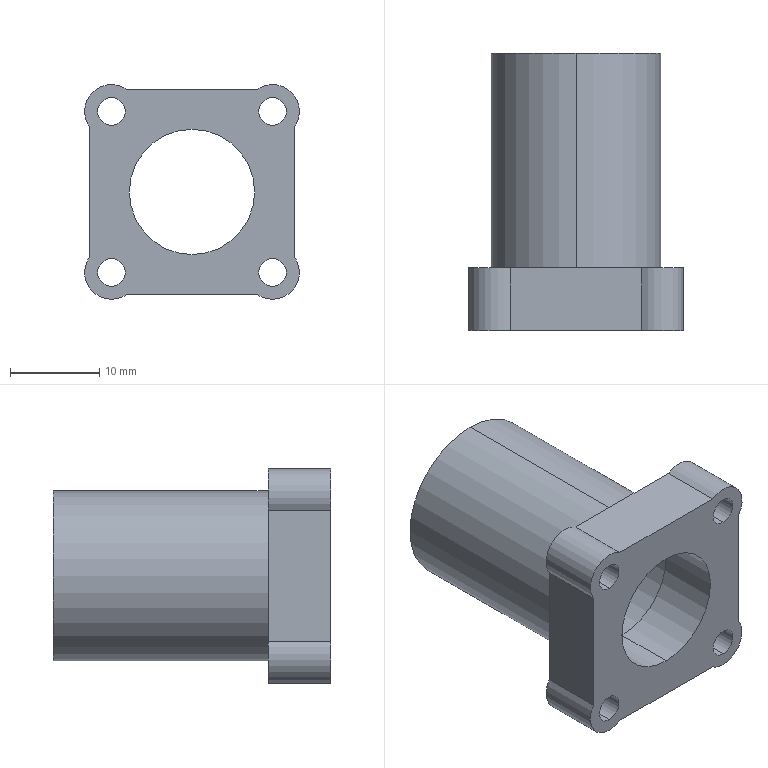Part | SolidWorks | features Extrusion 1, ICE 1 | 1 solid | 28 faces | box 24 x 31 x 24 mm | volume 4448 mm3 | cylinder 20 | plane 8 | commonest cylinder face diameters 3.1 x8 6 x6 14 x2 16 x2 19 x2
STEP:
#1=CARTESIAN_POINT('',(0.,31.,-8.));
#2=VERTEX_POINT('',#1);
#3=CARTESIAN_POINT('',(0.,31.,8.));
#4=VERTEX_POINT('',#3);
#5=CARTESIAN_POINT('',(0.,31.,0.));
#6=DIRECTION('',(0.,1.,0.));
#7=DIRECTION('',(0.,0.,1.));
#8=AXIS2_PLACEMENT_3D('',#5,#6,#7);
#9=CIRCLE('',#8,8.);
#10=EDGE_CURVE('',#2,#4,#9,.T.);
#11=ORIENTED_EDGE('',*,*,#10,.T.);
#12=CARTESIAN_POINT('',(0.,7.,8.));
#13=VERTEX_POINT('',#12);
#14=CARTESIAN_POINT('',(0.,31.,8.));
#15=DIRECTION('',(0.,-1.,0.));
#16=VECTOR('',#15,1000.);
#17=LINE('',#14,#16);
#18=EDGE_CURVE('',#4,#13,#17,.T.);
#19=ORIENTED_EDGE('',*,*,#18,.T.);
#20=CARTESIAN_POINT('',(0.,7.,-8.));
#21=VERTEX_POINT('',#20);
#22=CARTESIAN_POINT('',(0.,7.,0.));
#23=DIRECTION('',(0.,-1.,0.));
#24=DIRECTION('',(0.,0.,1.));
#25=AXIS2_PLACEMENT_3D('',#22,#23,#24);
#26=CIRCLE('',#25,8.);
#27=EDGE_CURVE('',#13,#21,#26,.T.);
#28=ORIENTED_EDGE('',*,*,#27,.T.);
#29=CARTESIAN_POINT('',(0.,31.,-8.));
#30=DIRECTION('',(0.,-1.,0.));
#31=VECTOR('',#30,1000.);
#32=LINE('',#29,#31);
#33=EDGE_CURVE('',#2,#21,#32,.T.);
#34=ORIENTED_EDGE('',*,*,#33,.F.);
#35=EDGE_LOOP('',(#11,#19,#28,#34));
#36=FACE_OUTER_BOUND('',#35,.T.);
#37=CARTESIAN_POINT('',(0.,31.,0.));
#38=DIRECTION('',(0.,-1.,0.));
#39=DIRECTION('',(0.,0.,-1.));
#40=AXIS2_PLACEMENT_3D('',#37,#38,#39);
#41=CYLINDRICAL_SURFACE('',#40,8.);
#42=ADVANCED_FACE('',(#36),#41,.F.);
#43=CARTESIAN_POINT('',(0.,31.,9.5));
#44=VERTEX_POINT('',#43);
#45=CARTESIAN_POINT('',(0.,31.,-9.5));
#46=VERTEX_POINT('',#45);
#47=CARTESIAN_POINT('',(0.,31.,0.));
#48=DIRECTION('',(0.,1.,0.));
#49=DIRECTION('',(0.,0.,1.));
#50=AXIS2_PLACEMENT_3D('',#47,#48,#49);
#51=CIRCLE('',#50,9.5);
#52=EDGE_CURVE('',#44,#46,#51,.T.);
#53=ORIENTED_EDGE('',*,*,#52,.F.);
#54=CARTESIAN_POINT('',(0.,7.,9.5));
#55=VERTEX_POINT('',#54);
#56=CARTESIAN_POINT('',(0.,31.,9.5));
#57=DIRECTION('',(0.,-1.,0.));
#58=VECTOR('',#57,1000.);
#59=LINE('',#56,#58);
#60=EDGE_CURVE('',#44,#55,#59,.T.);
#61=ORIENTED_EDGE('',*,*,#60,.T.);
#62=CARTESIAN_POINT('',(0.,7.,-9.5));
#63=VERTEX_POINT('',#62);
#64=CARTESIAN_POINT('',(0.,7.,0.));
#65=DIRECTION('',(0.,1.,0.));
#66=DIRECTION('',(0.,0.,1.));
#67=AXIS2_PLACEMENT_3D('',#64,#65,#66);
#68=CIRCLE('',#67,9.5);
#69=EDGE_CURVE('',#55,#63,#68,.T.);
#70=ORIENTED_EDGE('',*,*,#69,.T.);
#71=CARTESIAN_POINT('',(0.,31.,-9.5));
#72=DIRECTION('',(0.,-1.,0.));
#73=VECTOR('',#72,1000.);
#74=LINE('',#71,#73);
#75=EDGE_CURVE('',#46,#63,#74,.T.);
#76=ORIENTED_EDGE('',*,*,#75,.F.);
#77=EDGE_LOOP('',(#53,#61,#70,#76));
#78=FACE_OUTER_BOUND('',#77,.T.);
#79=CARTESIAN_POINT('',(0.,31.,0.));
#80=DIRECTION('',(0.,-1.,0.));
#81=DIRECTION('',(0.,0.,-1.));
#82=AXIS2_PLACEMENT_3D('',#79,#80,#81);
#83=CYLINDRICAL_SURFACE('',#82,9.5);
#84=ADVANCED_FACE('',(#78),#83,.T.);
#85=CARTESIAN_POINT('',(9.,7.,7.45));
#86=VERTEX_POINT('',#85);
#87=CARTESIAN_POINT('',(9.,7.,10.55));
#88=VERTEX_POINT('',#87);
#89=CARTESIAN_POINT('',(9.,7.,9.));
#90=DIRECTION('',(0.,1.,0.));
#91=DIRECTION('',(0.,0.,1.));
#92=AXIS2_PLACEMENT_3D('',#89,#90,#91);
#93=CIRCLE('',#92,1.55);
#94=EDGE_CURVE('',#86,#88,#93,.T.);
#95=ORIENTED_EDGE('',*,*,#94,.T.);
#96=CARTESIAN_POINT('',(9.,0.,10.55));
#97=VERTEX_POINT('',#96);
#98=CARTESIAN_POINT('',(9.,7.,10.55));
#99=DIRECTION('',(0.,-1.,0.));
#100=VECTOR('',#99,1000.);
#101=LINE('',#98,#100);
#102=EDGE_CURVE('',#88,#97,#101,.T.);
#103=ORIENTED_EDGE('',*,*,#102,.T.);
#104=CARTESIAN_POINT('',(9.,0.,7.45));
#105=VERTEX_POINT('',#104);
#106=CARTESIAN_POINT('',(9.,0.,9.));
#107=DIRECTION('',(0.,1.,0.));
#108=DIRECTION('',(0.,0.,1.));
#109=AXIS2_PLACEMENT_3D('',#106,#107,#108);
#110=CIRCLE('',#109,1.55);
#111=EDGE_CURVE('',#105,#97,#110,.T.);
#112=ORIENTED_EDGE('',*,*,#111,.F.);
#113=CARTESIAN_POINT('',(9.,7.,7.45));
#114=DIRECTION('',(0.,-1.,0.));
#115=VECTOR('',#114,1000.);
#116=LINE('',#113,#115);
#117=EDGE_CURVE('',#86,#105,#116,.T.);
#118=ORIENTED_EDGE('',*,*,#117,.F.);
#119=EDGE_LOOP('',(#95,#103,#112,#118));
#120=FACE_OUTER_BOUND('',#119,.T.);
#121=CARTESIAN_POINT('',(9.,7.,9.));
#122=DIRECTION('',(0.,-1.,0.));
#123=DIRECTION('',(0.,0.,-1.));
#124=AXIS2_PLACEMENT_3D('',#121,#122,#123);
#125=CYLINDRICAL_SURFACE('',#124,1.55);
#126=ADVANCED_FACE('',(#120),#125,.F.);
#127=CARTESIAN_POINT('',(0.,7.,-7.));
#128=VERTEX_POINT('',#127);
#129=CARTESIAN_POINT('',(0.,7.,7.));
#130=VERTEX_POINT('',#129);
#131=CARTESIAN_POINT('',(0.,7.,0.));
#132=DIRECTION('',(0.,1.,0.));
#133=DIRECTION('',(0.,0.,1.));
#134=AXIS2_PLACEMENT_3D('',#131,#132,#133);
#135=CIRCLE('',#134,7.);
#136=EDGE_CURVE('',#128,#130,#135,.T.);
#137=ORIENTED_EDGE('',*,*,#136,.T.);
#138=CARTESIAN_POINT('',(0.,0.,7.));
#139=VERTEX_POINT('',#138);
#140=CARTESIAN_POINT('',(0.,7.,7.));
#141=DIRECTION('',(0.,-1.,0.));
#142=VECTOR('',#141,1000.);
#143=LINE('',#140,#142);
#144=EDGE_CURVE('',#130,#139,#143,.T.);
#145=ORIENTED_EDGE('',*,*,#144,.T.);
#146=CARTESIAN_POINT('',(0.,0.,-7.));
#147=VERTEX_POINT('',#146);
#148=CARTESIAN_POINT('',(0.,0.,0.));
#149=DIRECTION('',(0.,1.,0.));
#150=DIRECTION('',(0.,0.,1.));
#151=AXIS2_PLACEMENT_3D('',#148,#149,#150);
#152=CIRCLE('',#151,7.);
#153=EDGE_CURVE('',#147,#139,#152,.T.);
#154=ORIENTED_EDGE('',*,*,#153,.F.);
#155=CARTESIAN_POINT('',(0.,7.,-7.));
#156=DIRECTION('',(0.,-1.,0.));
#157=VECTOR('',#156,1000.);
#158=LINE('',#155,#157);
#159=EDGE_CURVE('',#128,#147,#158,.T.);
#160=ORIENTED_EDGE('',*,*,#159,.F.);
#161=EDGE_LOOP('',(#137,#145,#154,#160));
#162=FACE_OUTER_BOUND('',#161,.T.);
#163=CARTESIAN_POINT('',(0.,7.,0.));
#164=DIRECTION('',(0.,-1.,0.));
#165=DIRECTION('',(0.,0.,-1.));
#166=AXIS2_PLACEMENT_3D('',#163,#164,#165);
#167=CYLINDRICAL_SURFACE('',#166,7.);
#168=ADVANCED_FACE('',(#162),#167,.F.);
#169=CARTESIAN_POINT('',(-9.,7.,7.45));
#170=VERTEX_POINT('',#169);
#171=CARTESIAN_POINT('',(-9.,7.,10.55));
#172=VERTEX_POINT('',#171);
#173=CARTESIAN_POINT('',(-9.,7.,9.));
#174=DIRECTION('',(0.,1.,0.));
#175=DIRECTION('',(0.,0.,1.));
#176=AXIS2_PLACEMENT_3D('',#173,#174,#175);
#177=CIRCLE('',#176,1.55);
#178=EDGE_CURVE('',#170,#172,#177,.T.);
#179=ORIENTED_EDGE('',*,*,#178,.T.);
#180=CARTESIAN_POINT('',(-9.,0.,10.55));
#181=VERTEX_POINT('',#180);
#182=CARTESIAN_POINT('',(-9.,7.,10.55));
#183=DIRECTION('',(0.,-1.,0.));
#184=VECTOR('',#183,1000.);
#185=LINE('',#182,#184);
#186=EDGE_CURVE('',#172,#181,#185,.T.);
#187=ORIENTED_EDGE('',*,*,#186,.T.);
#188=CARTESIAN_POINT('',(-9.,0.,7.45));
#189=VERTEX_POINT('',#188);
#190=CARTESIAN_POINT('',(-9.,0.,9.));
#191=DIRECTION('',(0.,1.,0.));
#192=DIRECTION('',(0.,0.,1.));
#193=AXIS2_PLACEMENT_3D('',#190,#191,#192);
#194=CIRCLE('',#193,1.55);
#195=EDGE_CURVE('',#189,#181,#194,.T.);
#196=ORIENTED_EDGE('',*,*,#195,.F.);
#197=CARTESIAN_POINT('',(-9.,7.,7.45));
#198=DIRECTION('',(0.,-1.,0.));
#199=VECTOR('',#198,1000.);
#200=LINE('',#197,#199);
#201=EDGE_CURVE('',#170,#189,#200,.T.);
#202=ORIENTED_EDGE('',*,*,#201,.F.);
#203=EDGE_LOOP('',(#179,#187,#196,#202));
#204=FACE_OUTER_BOUND('',#203,.T.);
#205=CARTESIAN_POINT('',(-9.,7.,9.));
#206=DIRECTION('',(0.,-1.,0.));
#207=DIRECTION('',(0.,0.,-1.));
#208=AXIS2_PLACEMENT_3D('',#205,#206,#207);
#209=CYLINDRICAL_SURFACE('',#208,1.55);
#210=ADVANCED_FACE('',(#204),#209,.F.);
#211=CARTESIAN_POINT('',(-9.,7.,-10.55));
#212=VERTEX_POINT('',#211);
#213=CARTESIAN_POINT('',(-9.,7.,-7.45));
#214=VERTEX_POINT('',#213);
#215=CARTESIAN_POINT('',(-9.,7.,-9.));
#216=DIRECTION('',(0.,1.,0.));
#217=DIRECTION('',(0.,0.,1.));
#218=AXIS2_PLACEMENT_3D('',#215,#216,#217);
#219=CIRCLE('',#218,1.55);
#220=EDGE_CURVE('',#212,#214,#219,.T.);
#221=ORIENTED_EDGE('',*,*,#220,.T.);
#222=CARTESIAN_POINT('',(-9.,0.,-7.45));
#223=VERTEX_POINT('',#222);
#224=CARTESIAN_POINT('',(-9.,7.,-7.45));
#225=DIRECTION('',(0.,-1.,0.));
#226=VECTOR('',#225,1000.);
#227=LINE('',#224,#226);
#228=EDGE_CURVE('',#214,#223,#227,.T.);
#229=ORIENTED_EDGE('',*,*,#228,.T.);
#230=CARTESIAN_POINT('',(-9.,0.,-10.55));
#231=VERTEX_POINT('',#230);
#232=CARTESIAN_POINT('',(-9.,0.,-9.));
#233=DIRECTION('',(0.,1.,0.));
#234=DIRECTION('',(0.,0.,1.));
#235=AXIS2_PLACEMENT_3D('',#232,#233,#234);
#236=CIRCLE('',#235,1.55);
#237=EDGE_CURVE('',#231,#223,#236,.T.);
#238=ORIENTED_EDGE('',*,*,#237,.F.);
#239=CARTESIAN_POINT('',(-9.,7.,-10.55));
#240=DIRECTION('',(0.,-1.,0.));
#241=VECTOR('',#240,1000.);
#242=LINE('',#239,#241);
#243=EDGE_CURVE('',#212,#231,#242,.T.);
#244=ORIENTED_EDGE('',*,*,#243,.F.);
#245=EDGE_LOOP('',(#221,#229,#238,#244));
#246=FACE_OUTER_BOUND('',#245,.T.);
#247=CARTESIAN_POINT('',(-9.,7.,-9.));
#248=DIRECTION('',(0.,-1.,0.));
#249=DIRECTION('',(0.,0.,-1.));
#250=AXIS2_PLACEMENT_3D('',#247,#248,#249);
#251=CYLINDRICAL_SURFACE('',#250,1.55);
#252=ADVANCED_FACE('',(#246),#251,.F.);
#253=CARTESIAN_POINT('',(9.,7.,-10.55));
#254=VERTEX_POINT('',#253);
#255=CARTESIAN_POINT('',(9.,7.,-7.45));
#256=VERTEX_POINT('',#255);
#257=CARTESIAN_POINT('',(9.,7.,-9.));
#258=DIRECTION('',(0.,1.,0.));
#259=DIRECTION('',(0.,0.,1.));
#260=AXIS2_PLACEMENT_3D('',#257,#258,#259);
#261=CIRCLE('',#260,1.55);
#262=EDGE_CURVE('',#254,#256,#261,.T.);
#263=ORIENTED_EDGE('',*,*,#262,.T.);
#264=CARTESIAN_POINT('',(9.,0.,-7.45));
#265=VERTEX_POINT('',#264);
#266=CARTESIAN_POINT('',(9.,7.,-7.45));
#267=DIRECTION('',(0.,-1.,0.));
#268=VECTOR('',#267,1000.);
#269=LINE('',#266,#268);
#270=EDGE_CURVE('',#256,#265,#269,.T.);
#271=ORIENTED_EDGE('',*,*,#270,.T.);
#272=CARTESIAN_POINT('',(9.,0.,-10.55));
#273=VERTEX_POINT('',#272);
#274=CARTESIAN_POINT('',(9.,0.,-9.));
#275=DIRECTION('',(0.,1.,0.));
#276=DIRECTION('',(0.,0.,1.));
#277=AXIS2_PLACEMENT_3D('',#274,#275,#276);
#278=CIRCLE('',#277,1.55);
#279=EDGE_CURVE('',#273,#265,#278,.T.);
#280=ORIENTED_EDGE('',*,*,#279,.F.);
#281=CARTESIAN_POINT('',(9.,7.,-10.55));
#282=DIRECTION('',(0.,-1.,0.));
#283=VECTOR('',#282,1000.);
#284=LINE('',#281,#283);
#285=EDGE_CURVE('',#254,#273,#284,.T.);
#286=ORIENTED_EDGE('',*,*,#285,.F.);
#287=EDGE_LOOP('',(#263,#271,#280,#286));
#288=FACE_OUTER_BOUND('',#287,.T.);
#289=CARTESIAN_POINT('',(9.,7.,-9.));
#290=DIRECTION('',(0.,-1.,0.));
#291=DIRECTION('',(0.,0.,-1.));
#292=AXIS2_PLACEMENT_3D('',#289,#290,#291);
#293=CYLINDRICAL_SURFACE('',#292,1.55);
#294=ADVANCED_FACE('',(#288),#293,.F.);
#295=CARTESIAN_POINT('',(-9.,7.,-12.));
#296=VERTEX_POINT('',#295);
#297=CARTESIAN_POINT('',(-11.5,7.,-7.342));
#298=VERTEX_POINT('',#297);
#299=CARTESIAN_POINT('',(-9.,7.,-9.));
#300=DIRECTION('',(0.,1.,0.));
#301=DIRECTION('',(0.,0.,1.));
#302=AXIS2_PLACEMENT_3D('',#299,#300,#301);
#303=CIRCLE('',#302,3.);
#304=EDGE_CURVE('',#296,#298,#303,.T.);
#305=ORIENTED_EDGE('',*,*,#304,.F.);
#306=CARTESIAN_POINT('',(-9.,0.,-12.));
#307=VERTEX_POINT('',#306);
#308=CARTESIAN_POINT('',(-9.,7.,-12.));
#309=DIRECTION('',(0.,-1.,0.));
#310=VECTOR('',#309,1000.);
#311=LINE('',#308,#310);
#312=EDGE_CURVE('',#296,#307,#311,.T.);
#313=ORIENTED_EDGE('',*,*,#312,.T.);
#314=CARTESIAN_POINT('',(-11.5,0.,-7.342));
#315=VERTEX_POINT('',#314);
#316=CARTESIAN_POINT('',(-9.,0.,-9.));
#317=DIRECTION('',(0.,1.,0.));
#318=DIRECTION('',(0.,0.,1.));
#319=AXIS2_PLACEMENT_3D('',#316,#317,#318);
#320=CIRCLE('',#319,3.);
#321=EDGE_CURVE('',#307,#315,#320,.T.);
#322=ORIENTED_EDGE('',*,*,#321,.T.);
#323=CARTESIAN_POINT('',(-11.5,7.,-7.342));
#324=DIRECTION('',(0.,-1.,0.));
#325=VECTOR('',#324,1000.);
#326=LINE('',#323,#325);
#327=EDGE_CURVE('',#298,#315,#326,.T.);
#328=ORIENTED_EDGE('',*,*,#327,.F.);
#329=EDGE_LOOP('',(#305,#313,#322,#328));
#330=FACE_OUTER_BOUND('',#329,.T.);
#331=CARTESIAN_POINT('',(-9.,7.,-9.));
#332=DIRECTION('',(0.,-1.,0.));
#333=DIRECTION('',(0.,0.,-1.));
#334=AXIS2_PLACEMENT_3D('',#331,#332,#333);
#335=CYLINDRICAL_SURFACE('',#334,3.);
#336=ADVANCED_FACE('',(#330),#335,.T.);
#337=CARTESIAN_POINT('',(9.,7.,-12.));
#338=VERTEX_POINT('',#337);
#339=CARTESIAN_POINT('',(7.342,7.,-11.5));
#340=VERTEX_POINT('',#339);
#341=CARTESIAN_POINT('',(9.,7.,-9.));
#342=DIRECTION('',(0.,1.,0.));
#343=DIRECTION('',(0.,0.,1.));
#344=AXIS2_PLACEMENT_3D('',#341,#342,#343);
#345=CIRCLE('',#344,3.);
#346=EDGE_CURVE('',#338,#340,#345,.T.);
#347=ORIENTED_EDGE('',*,*,#346,.F.);
#348=CARTESIAN_POINT('',(9.,0.,-12.));
#349=VERTEX_POINT('',#348);
#350=CARTESIAN_POINT('',(9.,7.,-12.));
#351=DIRECTION('',(0.,-1.,0.));
#352=VECTOR('',#351,1000.);
#353=LINE('',#350,#352);
#354=EDGE_CURVE('',#338,#349,#353,.T.);
#355=ORIENTED_EDGE('',*,*,#354,.T.);
#356=CARTESIAN_POINT('',(7.342,0.,-11.5));
#357=VERTEX_POINT('',#356);
#358=CARTESIAN_POINT('',(9.,0.,-9.));
#359=DIRECTION('',(0.,1.,0.));
#360=DIRECTION('',(0.,0.,1.));
#361=AXIS2_PLACEMENT_3D('',#358,#359,#360);
#362=CIRCLE('',#361,3.);
#363=EDGE_CURVE('',#349,#357,#362,.T.);
#364=ORIENTED_EDGE('',*,*,#363,.T.);
#365=CARTESIAN_POINT('',(7.342,7.,-11.5));
#366=DIRECTION('',(0.,-1.,0.));
#367=VECTOR('',#366,1000.);
#368=LINE('',#365,#367);
#369=EDGE_CURVE('',#340,#357,#368,.T.);
#370=ORIENTED_EDGE('',*,*,#369,.F.);
#371=EDGE_LOOP('',(#347,#355,#364,#370));
#372=FACE_OUTER_BOUND('',#371,.T.);
#373=CARTESIAN_POINT('',(9.,7.,-9.));
#374=DIRECTION('',(0.,-1.,0.));
#375=DIRECTION('',(0.,0.,-1.));
#376=AXIS2_PLACEMENT_3D('',#373,#374,#375);
#377=CYLINDRICAL_SURFACE('',#376,3.);
#378=ADVANCED_FACE('',(#372),#377,.T.);
#379=ORIENTED_EDGE('',*,*,#136,.F.);
#380=CARTESIAN_POINT('',(0.,7.,0.));
#381=DIRECTION('',(0.,1.,0.));
#382=DIRECTION('',(0.,0.,1.));
#383=AXIS2_PLACEMENT_3D('',#380,#381,#382);
#384=CIRCLE('',#383,7.);
#385=EDGE_CURVE('',#130,#128,#384,.T.);
#386=ORIENTED_EDGE('',*,*,#385,.F.);
#387=EDGE_LOOP('',(#379,#386));
#388=FACE_BOUND('',#387,.T.);
#389=CARTESIAN_POINT('',(0.,7.,0.));
#390=DIRECTION('',(0.,-1.,0.));
#391=DIRECTION('',(0.,0.,1.));
#392=AXIS2_PLACEMENT_3D('',#389,#390,#391);
#393=CIRCLE('',#392,8.);
#394=EDGE_CURVE('',#21,#13,#393,.T.);
#395=ORIENTED_EDGE('',*,*,#394,.F.);
#396=ORIENTED_EDGE('',*,*,#27,.F.);
#397=EDGE_LOOP('',(#395,#396));
#398=FACE_OUTER_BOUND('',#397,.T.);
#399=CARTESIAN_POINT('',(0.,7.,0.));
#400=DIRECTION('',(0.,1.,0.));
#401=DIRECTION('',(0.,0.,1.));
#402=AXIS2_PLACEMENT_3D('',#399,#400,#401);
#403=PLANE('',#402);
#404=ADVANCED_FACE('',(#388,#398),#403,.T.);
#405=CARTESIAN_POINT('',(7.342,0.,11.5));
#406=VERTEX_POINT('',#405);
#407=CARTESIAN_POINT('',(-7.342,0.,11.5));
#408=VERTEX_POINT('',#407);
#409=CARTESIAN_POINT('',(0.,0.,11.5));
#410=DIRECTION('',(-1.,0.,0.));
#411=VECTOR('',#410,1000.);
#412=LINE('',#409,#411);
#413=EDGE_CURVE('',#406,#408,#412,.T.);
#414=ORIENTED_EDGE('',*,*,#413,.F.);
#415=CARTESIAN_POINT('',(7.342,7.,11.5));
#416=VERTEX_POINT('',#415);
#417=CARTESIAN_POINT('',(7.342,7.,11.5));
#418=DIRECTION('',(0.,-1.,0.));
#419=VECTOR('',#418,1000.);
#420=LINE('',#417,#419);
#421=EDGE_CURVE('',#416,#406,#420,.T.);
#422=ORIENTED_EDGE('',*,*,#421,.F.);
#423=CARTESIAN_POINT('',(-7.342,7.,11.5));
#424=VERTEX_POINT('',#423);
#425=CARTESIAN_POINT('',(0.,7.,11.5));
#426=DIRECTION('',(-1.,0.,0.));
#427=VECTOR('',#426,1000.);
#428=LINE('',#425,#427);
#429=EDGE_CURVE('',#416,#424,#428,.T.);
#430=ORIENTED_EDGE('',*,*,#429,.T.);
#431=CARTESIAN_POINT('',(-7.342,7.,11.5));
#432=DIRECTION('',(0.,-1.,0.));
#433=VECTOR('',#432,1000.);
#434=LINE('',#431,#433);
#435=EDGE_CURVE('',#424,#408,#434,.T.);
#436=ORIENTED_EDGE('',*,*,#435,.T.);
#437=EDGE_LOOP('',(#414,#422,#430,#436));
#438=FACE_OUTER_BOUND('',#437,.T.);
#439=CARTESIAN_POINT('',(0.,7.,11.5));
#440=DIRECTION('',(0.,0.,1.));
#441=DIRECTION('',(1.,0.,0.));
#442=AXIS2_PLACEMENT_3D('',#439,#440,#441);
#443=PLANE('',#442);
#444=ADVANCED_FACE('',(#438),#443,.T.);
#445=CARTESIAN_POINT('',(11.5,0.,7.342));
#446=VERTEX_POINT('',#445);
#447=CARTESIAN_POINT('',(9.,0.,9.));
#448=DIRECTION('',(0.,1.,0.));
#449=DIRECTION('',(0.,0.,1.));
#450=AXIS2_PLACEMENT_3D('',#447,#448,#449);
#451=CIRCLE('',#450,3.);
#452=EDGE_CURVE('',#406,#446,#451,.T.);
#453=ORIENTED_EDGE('',*,*,#452,.T.);
#454=CARTESIAN_POINT('',(11.5,7.,7.342));
#455=VERTEX_POINT('',#454);
#456=CARTESIAN_POINT('',(11.5,7.,7.342));
#457=DIRECTION('',(0.,-1.,0.));
#458=VECTOR('',#457,1000.);
#459=LINE('',#456,#458);
#460=EDGE_CURVE('',#455,#446,#459,.T.);
#461=ORIENTED_EDGE('',*,*,#460,.F.);
#462=CARTESIAN_POINT('',(9.,7.,9.));
#463=DIRECTION('',(0.,1.,0.));
#464=DIRECTION('',(0.,0.,1.));
#465=AXIS2_PLACEMENT_3D('',#462,#463,#464);
#466=CIRCLE('',#465,3.);
#467=EDGE_CURVE('',#416,#455,#466,.T.);
#468=ORIENTED_EDGE('',*,*,#467,.F.);
#469=ORIENTED_EDGE('',*,*,#421,.T.);
#470=EDGE_LOOP('',(#453,#461,#468,#469));
#471=FACE_OUTER_BOUND('',#470,.T.);
#472=CARTESIAN_POINT('',(9.,7.,9.));
#473=DIRECTION('',(0.,-1.,0.));
#474=DIRECTION('',(0.,0.,-1.));
#475=AXIS2_PLACEMENT_3D('',#472,#473,#474);
#476=CYLINDRICAL_SURFACE('',#475,3.);
#477=ADVANCED_FACE('',(#471),#476,.T.);
#478=CARTESIAN_POINT('',(11.5,0.,-7.342));
#479=VERTEX_POINT('',#478);
#480=CARTESIAN_POINT('',(11.5,0.,0.));
#481=DIRECTION('',(0.,0.,-1.));
#482=VECTOR('',#481,1000.);
#483=LINE('',#480,#482);
#484=EDGE_CURVE('',#446,#479,#483,.T.);
#485=ORIENTED_EDGE('',*,*,#484,.T.);
#486=CARTESIAN_POINT('',(11.5,7.,-7.342));
#487=VERTEX_POINT('',#486);
#488=CARTESIAN_POINT('',(11.5,7.,-7.342));
#489=DIRECTION('',(0.,-1.,0.));
#490=VECTOR('',#489,1000.);
#491=LINE('',#488,#490);
#492=EDGE_CURVE('',#487,#479,#491,.T.);
#493=ORIENTED_EDGE('',*,*,#492,.F.);
#494=CARTESIAN_POINT('',(11.5,7.,0.));
#495=DIRECTION('',(0.,0.,-1.));
#496=VECTOR('',#495,1000.);
#497=LINE('',#494,#496);
#498=EDGE_CURVE('',#455,#487,#497,.T.);
#499=ORIENTED_EDGE('',*,*,#498,.F.);
#500=ORIENTED_EDGE('',*,*,#460,.T.);
#501=EDGE_LOOP('',(#485,#493,#499,#500));
#502=FACE_OUTER_BOUND('',#501,.T.);
#503=CARTESIAN_POINT('',(11.5,7.,0.));
#504=DIRECTION('',(-1.,0.,0.));
#505=DIRECTION('',(0.,0.,1.));
#506=AXIS2_PLACEMENT_3D('',#503,#504,#505);
#507=PLANE('',#506);
#508=ADVANCED_FACE('',(#502),#507,.F.);
#509=ORIENTED_EDGE('',*,*,#354,.F.);
#510=CARTESIAN_POINT('',(9.,7.,-9.));
#511=DIRECTION('',(0.,1.,0.));
#512=DIRECTION('',(0.,0.,1.));
#513=AXIS2_PLACEMENT_3D('',#510,#511,#512);
#514=CIRCLE('',#513,3.);
#515=EDGE_CURVE('',#487,#338,#514,.T.);
#516=ORIENTED_EDGE('',*,*,#515,.F.);
#517=ORIENTED_EDGE('',*,*,#492,.T.);
#518=CARTESIAN_POINT('',(9.,0.,-9.));
#519=DIRECTION('',(0.,1.,0.));
#520=DIRECTION('',(0.,0.,1.));
#521=AXIS2_PLACEMENT_3D('',#518,#519,#520);
#522=CIRCLE('',#521,3.);
#523=EDGE_CURVE('',#479,#349,#522,.T.);
#524=ORIENTED_EDGE('',*,*,#523,.T.);
#525=EDGE_LOOP('',(#509,#516,#517,#524));
#526=FACE_OUTER_BOUND('',#525,.T.);
#527=CARTESIAN_POINT('',(9.,7.,-9.));
#528=DIRECTION('',(0.,-1.,0.));
#529=DIRECTION('',(0.,0.,-1.));
#530=AXIS2_PLACEMENT_3D('',#527,#528,#529);
#531=CYLINDRICAL_SURFACE('',#530,3.);
#532=ADVANCED_FACE('',(#526),#531,.T.);
#533=CARTESIAN_POINT('',(-7.342,0.,-11.5));
#534=VERTEX_POINT('',#533);
#535=CARTESIAN_POINT('',(0.,0.,-11.5));
#536=DIRECTION('',(1.,0.,0.));
#537=VECTOR('',#536,1000.);
#538=LINE('',#535,#537);
#539=EDGE_CURVE('',#534,#357,#538,.T.);
#540=ORIENTED_EDGE('',*,*,#539,.F.);
#541=CARTESIAN_POINT('',(-7.342,7.,-11.5));
#542=VERTEX_POINT('',#541);
#543=CARTESIAN_POINT('',(-7.342,7.,-11.5));
#544=DIRECTION('',(0.,-1.,0.));
#545=VECTOR('',#544,1000.);
#546=LINE('',#543,#545);
#547=EDGE_CURVE('',#542,#534,#546,.T.);
#548=ORIENTED_EDGE('',*,*,#547,.F.);
#549=CARTESIAN_POINT('',(0.,7.,-11.5));
#550=DIRECTION('',(1.,0.,0.));
#551=VECTOR('',#550,1000.);
#552=LINE('',#549,#551);
#553=EDGE_CURVE('',#542,#340,#552,.T.);
#554=ORIENTED_EDGE('',*,*,#553,.T.);
#555=ORIENTED_EDGE('',*,*,#369,.T.);
#556=EDGE_LOOP('',(#540,#548,#554,#555));
#557=FACE_OUTER_BOUND('',#556,.T.);
#558=CARTESIAN_POINT('',(0.,7.,-11.5));
#559=DIRECTION('',(0.,0.,-1.));
#560=DIRECTION('',(-1.,0.,0.));
#561=AXIS2_PLACEMENT_3D('',#558,#559,#560);
#562=PLANE('',#561);
#563=ADVANCED_FACE('',(#557),#562,.T.);
#564=ORIENTED_EDGE('',*,*,#312,.F.);
#565=CARTESIAN_POINT('',(-9.,7.,-9.));
#566=DIRECTION('',(0.,1.,0.));
#567=DIRECTION('',(0.,0.,1.));
#568=AXIS2_PLACEMENT_3D('',#565,#566,#567);
#569=CIRCLE('',#568,3.);
#570=EDGE_CURVE('',#542,#296,#569,.T.);
#571=ORIENTED_EDGE('',*,*,#570,.F.);
#572=ORIENTED_EDGE('',*,*,#547,.T.);
#573=CARTESIAN_POINT('',(-9.,0.,-9.));
#574=DIRECTION('',(0.,1.,0.));
#575=DIRECTION('',(0.,0.,1.));
#576=AXIS2_PLACEMENT_3D('',#573,#574,#575);
#577=CIRCLE('',#576,3.);
#578=EDGE_CURVE('',#534,#307,#577,.T.);
#579=ORIENTED_EDGE('',*,*,#578,.T.);
#580=EDGE_LOOP('',(#564,#571,#572,#579));
#581=FACE_OUTER_BOUND('',#580,.T.);
#582=CARTESIAN_POINT('',(-9.,7.,-9.));
#583=DIRECTION('',(0.,-1.,0.));
#584=DIRECTION('',(0.,0.,-1.));
#585=AXIS2_PLACEMENT_3D('',#582,#583,#584);
#586=CYLINDRICAL_SURFACE('',#585,3.);
#587=ADVANCED_FACE('',(#581),#586,.T.);
#588=CARTESIAN_POINT('',(-11.5,0.,7.342));
#589=VERTEX_POINT('',#588);
#590=CARTESIAN_POINT('',(-11.5,0.,0.));
#591=DIRECTION('',(0.,0.,1.));
#592=VECTOR('',#591,1000.);
#593=LINE('',#590,#592);
#594=EDGE_CURVE('',#315,#589,#593,.T.);
#595=ORIENTED_EDGE('',*,*,#594,.T.);
#596=CARTESIAN_POINT('',(-11.5,7.,7.342));
#597=VERTEX_POINT('',#596);
#598=CARTESIAN_POINT('',(-11.5,7.,7.342));
#599=DIRECTION('',(0.,-1.,0.));
#600=VECTOR('',#599,1000.);
#601=LINE('',#598,#600);
#602=EDGE_CURVE('',#597,#589,#601,.T.);
#603=ORIENTED_EDGE('',*,*,#602,.F.);
#604=CARTESIAN_POINT('',(-11.5,7.,0.));
#605=DIRECTION('',(0.,0.,1.));
#606=VECTOR('',#605,1000.);
#607=LINE('',#604,#606);
#608=EDGE_CURVE('',#298,#597,#607,.T.);
#609=ORIENTED_EDGE('',*,*,#608,.F.);
#610=ORIENTED_EDGE('',*,*,#327,.T.);
#611=EDGE_LOOP('',(#595,#603,#609,#610));
#612=FACE_OUTER_BOUND('',#611,.T.);
#613=CARTESIAN_POINT('',(-11.5,7.,0.));
#614=DIRECTION('',(1.,0.,0.));
#615=DIRECTION('',(0.,0.,-1.));
#616=AXIS2_PLACEMENT_3D('',#613,#614,#615);
#617=PLANE('',#616);
#618=ADVANCED_FACE('',(#612),#617,.F.);
#619=ORIENTED_EDGE('',*,*,#270,.F.);
#620=CARTESIAN_POINT('',(9.,7.,-9.));
#621=DIRECTION('',(0.,1.,0.));
#622=DIRECTION('',(0.,0.,1.));
#623=AXIS2_PLACEMENT_3D('',#620,#621,#622);
#624=CIRCLE('',#623,1.55);
#625=EDGE_CURVE('',#256,#254,#624,.T.);
#626=ORIENTED_EDGE('',*,*,#625,.T.);
#627=ORIENTED_EDGE('',*,*,#285,.T.);
#628=CARTESIAN_POINT('',(9.,0.,-9.));
#629=DIRECTION('',(0.,1.,0.));
#630=DIRECTION('',(0.,0.,1.));
#631=AXIS2_PLACEMENT_3D('',#628,#629,#630);
#632=CIRCLE('',#631,1.55);
#633=EDGE_CURVE('',#265,#273,#632,.T.);
#634=ORIENTED_EDGE('',*,*,#633,.F.);
#635=EDGE_LOOP('',(#619,#626,#627,#634));
#636=FACE_OUTER_BOUND('',#635,.T.);
#637=CARTESIAN_POINT('',(9.,7.,-9.));
#638=DIRECTION('',(0.,-1.,0.));
#639=DIRECTION('',(0.,0.,-1.));
#640=AXIS2_PLACEMENT_3D('',#637,#638,#639);
#641=CYLINDRICAL_SURFACE('',#640,1.55);
#642=ADVANCED_FACE('',(#636),#641,.F.);
#643=ORIENTED_EDGE('',*,*,#228,.F.);
#644=CARTESIAN_POINT('',(-9.,7.,-9.));
#645=DIRECTION('',(0.,1.,0.));
#646=DIRECTION('',(0.,0.,1.));
#647=AXIS2_PLACEMENT_3D('',#644,#645,#646);
#648=CIRCLE('',#647,1.55);
#649=EDGE_CURVE('',#214,#212,#648,.T.);
#650=ORIENTED_EDGE('',*,*,#649,.T.);
#651=ORIENTED_EDGE('',*,*,#243,.T.);
#652=CARTESIAN_POINT('',(-9.,0.,-9.));
#653=DIRECTION('',(0.,1.,0.));
#654=DIRECTION('',(0.,0.,1.));
#655=AXIS2_PLACEMENT_3D('',#652,#653,#654);
#656=CIRCLE('',#655,1.55);
#657=EDGE_CURVE('',#223,#231,#656,.T.);
#658=ORIENTED_EDGE('',*,*,#657,.F.);
#659=EDGE_LOOP('',(#643,#650,#651,#658));
#660=FACE_OUTER_BOUND('',#659,.T.);
#661=CARTESIAN_POINT('',(-9.,7.,-9.));
#662=DIRECTION('',(0.,-1.,0.));
#663=DIRECTION('',(0.,0.,-1.));
#664=AXIS2_PLACEMENT_3D('',#661,#662,#663);
#665=CYLINDRICAL_SURFACE('',#664,1.55);
#666=ADVANCED_FACE('',(#660),#665,.F.);
#667=ORIENTED_EDGE('',*,*,#186,.F.);
#668=CARTESIAN_POINT('',(-9.,7.,9.));
#669=DIRECTION('',(0.,1.,0.));
#670=DIRECTION('',(0.,0.,1.));
#671=AXIS2_PLACEMENT_3D('',#668,#669,#670);
#672=CIRCLE('',#671,1.55);
#673=EDGE_CURVE('',#172,#170,#672,.T.);
#674=ORIENTED_EDGE('',*,*,#673,.T.);
#675=ORIENTED_EDGE('',*,*,#201,.T.);
#676=CARTESIAN_POINT('',(-9.,0.,9.));
#677=DIRECTION('',(0.,1.,0.));
#678=DIRECTION('',(0.,0.,1.));
#679=AXIS2_PLACEMENT_3D('',#676,#677,#678);
#680=CIRCLE('',#679,1.55);
#681=EDGE_CURVE('',#181,#189,#680,.T.);
#682=ORIENTED_EDGE('',*,*,#681,.F.);
#683=EDGE_LOOP('',(#667,#674,#675,#682));
#684=FACE_OUTER_BOUND('',#683,.T.);
#685=CARTESIAN_POINT('',(-9.,7.,9.));
#686=DIRECTION('',(0.,-1.,0.));
#687=DIRECTION('',(0.,0.,-1.));
#688=AXIS2_PLACEMENT_3D('',#685,#686,#687);
#689=CYLINDRICAL_SURFACE('',#688,1.55);
#690=ADVANCED_FACE('',(#684),#689,.F.);
#691=CARTESIAN_POINT('',(-9.,0.,9.));
#692=DIRECTION('',(0.,1.,0.));
#693=DIRECTION('',(0.,0.,1.));
#694=AXIS2_PLACEMENT_3D('',#691,#692,#693);
#695=CIRCLE('',#694,3.);
#696=EDGE_CURVE('',#589,#408,#695,.T.);
#697=ORIENTED_EDGE('',*,*,#696,.T.);
#698=ORIENTED_EDGE('',*,*,#435,.F.);
#699=CARTESIAN_POINT('',(-9.,7.,9.));
#700=DIRECTION('',(0.,1.,0.));
#701=DIRECTION('',(0.,0.,1.));
#702=AXIS2_PLACEMENT_3D('',#699,#700,#701);
#703=CIRCLE('',#702,3.);
#704=EDGE_CURVE('',#597,#424,#703,.T.);
#705=ORIENTED_EDGE('',*,*,#704,.F.);
#706=ORIENTED_EDGE('',*,*,#602,.T.);
#707=EDGE_LOOP('',(#697,#698,#705,#706));
#708=FACE_OUTER_BOUND('',#707,.T.);
#709=CARTESIAN_POINT('',(-9.,7.,9.));
#710=DIRECTION('',(0.,-1.,0.));
#711=DIRECTION('',(0.,0.,-1.));
#712=AXIS2_PLACEMENT_3D('',#709,#710,#711);
#713=CYLINDRICAL_SURFACE('',#712,3.);
#714=ADVANCED_FACE('',(#708),#713,.T.);
#715=ORIENTED_EDGE('',*,*,#144,.F.);
#716=ORIENTED_EDGE('',*,*,#385,.T.);
#717=ORIENTED_EDGE('',*,*,#159,.T.);
#718=CARTESIAN_POINT('',(0.,0.,0.));
#719=DIRECTION('',(0.,1.,0.));
#720=DIRECTION('',(0.,0.,1.));
#721=AXIS2_PLACEMENT_3D('',#718,#719,#720);
#722=CIRCLE('',#721,7.);
#723=EDGE_CURVE('',#139,#147,#722,.T.);
#724=ORIENTED_EDGE('',*,*,#723,.F.);
#725=EDGE_LOOP('',(#715,#716,#717,#724));
#726=FACE_OUTER_BOUND('',#725,.T.);
#727=CARTESIAN_POINT('',(0.,7.,0.));
#728=DIRECTION('',(0.,-1.,0.));
#729=DIRECTION('',(0.,0.,-1.));
#730=AXIS2_PLACEMENT_3D('',#727,#728,#729);
#731=CYLINDRICAL_SURFACE('',#730,7.);
#732=ADVANCED_FACE('',(#726),#731,.F.);
#733=ORIENTED_EDGE('',*,*,#102,.F.);
#734=CARTESIAN_POINT('',(9.,7.,9.));
#735=DIRECTION('',(0.,1.,0.));
#736=DIRECTION('',(0.,0.,1.));
#737=AXIS2_PLACEMENT_3D('',#734,#735,#736);
#738=CIRCLE('',#737,1.55);
#739=EDGE_CURVE('',#88,#86,#738,.T.);
#740=ORIENTED_EDGE('',*,*,#739,.T.);
#741=ORIENTED_EDGE('',*,*,#117,.T.);
#742=CARTESIAN_POINT('',(9.,0.,9.));
#743=DIRECTION('',(0.,1.,0.));
#744=DIRECTION('',(0.,0.,1.));
#745=AXIS2_PLACEMENT_3D('',#742,#743,#744);
#746=CIRCLE('',#745,1.55);
#747=EDGE_CURVE('',#97,#105,#746,.T.);
#748=ORIENTED_EDGE('',*,*,#747,.F.);
#749=EDGE_LOOP('',(#733,#740,#741,#748));
#750=FACE_OUTER_BOUND('',#749,.T.);
#751=CARTESIAN_POINT('',(9.,7.,9.));
#752=DIRECTION('',(0.,-1.,0.));
#753=DIRECTION('',(0.,0.,-1.));
#754=AXIS2_PLACEMENT_3D('',#751,#752,#753);
#755=CYLINDRICAL_SURFACE('',#754,1.55);
#756=ADVANCED_FACE('',(#750),#755,.F.);
#757=CARTESIAN_POINT('',(0.,7.,0.));
#758=DIRECTION('',(0.,1.,0.));
#759=DIRECTION('',(0.,0.,1.));
#760=AXIS2_PLACEMENT_3D('',#757,#758,#759);
#761=CIRCLE('',#760,9.5);
#762=EDGE_CURVE('',#63,#55,#761,.T.);
#763=ORIENTED_EDGE('',*,*,#762,.F.);
#764=ORIENTED_EDGE('',*,*,#69,.F.);
#765=EDGE_LOOP('',(#763,#764));
#766=FACE_BOUND('',#765,.T.);
#767=ORIENTED_EDGE('',*,*,#429,.F.);
#768=ORIENTED_EDGE('',*,*,#467,.T.);
#769=ORIENTED_EDGE('',*,*,#498,.T.);
#770=ORIENTED_EDGE('',*,*,#515,.T.);
#771=ORIENTED_EDGE('',*,*,#346,.T.);
#772=ORIENTED_EDGE('',*,*,#553,.F.);
#773=ORIENTED_EDGE('',*,*,#570,.T.);
#774=ORIENTED_EDGE('',*,*,#304,.T.);
#775=ORIENTED_EDGE('',*,*,#608,.T.);
#776=ORIENTED_EDGE('',*,*,#704,.T.);
#777=EDGE_LOOP('',(#767,#768,#769,#770,#771,#772,#773,#774,#775,#776));
#778=FACE_OUTER_BOUND('',#777,.T.);
#779=ORIENTED_EDGE('',*,*,#178,.F.);
#780=ORIENTED_EDGE('',*,*,#673,.F.);
#781=EDGE_LOOP('',(#779,#780));
#782=FACE_BOUND('',#781,.T.);
#783=ORIENTED_EDGE('',*,*,#220,.F.);
#784=ORIENTED_EDGE('',*,*,#649,.F.);
#785=EDGE_LOOP('',(#783,#784));
#786=FACE_BOUND('',#785,.T.);
#787=ORIENTED_EDGE('',*,*,#262,.F.);
#788=ORIENTED_EDGE('',*,*,#625,.F.);
#789=EDGE_LOOP('',(#787,#788));
#790=FACE_BOUND('',#789,.T.);
#791=ORIENTED_EDGE('',*,*,#94,.F.);
#792=ORIENTED_EDGE('',*,*,#739,.F.);
#793=EDGE_LOOP('',(#791,#792));
#794=FACE_BOUND('',#793,.T.);
#795=CARTESIAN_POINT('',(0.,7.,0.));
#796=DIRECTION('',(0.,1.,0.));
#797=DIRECTION('',(0.,0.,1.));
#798=AXIS2_PLACEMENT_3D('',#795,#796,#797);
#799=PLANE('',#798);
#800=ADVANCED_FACE('',(#766,#778,#782,#786,#790,#794),#799,.T.);
#801=ORIENTED_EDGE('',*,*,#153,.T.);
#802=ORIENTED_EDGE('',*,*,#723,.T.);
#803=EDGE_LOOP('',(#801,#802));
#804=FACE_BOUND('',#803,.T.);
#805=ORIENTED_EDGE('',*,*,#413,.T.);
#806=ORIENTED_EDGE('',*,*,#696,.F.);
#807=ORIENTED_EDGE('',*,*,#594,.F.);
#808=ORIENTED_EDGE('',*,*,#321,.F.);
#809=ORIENTED_EDGE('',*,*,#578,.F.);
#810=ORIENTED_EDGE('',*,*,#539,.T.);
#811=ORIENTED_EDGE('',*,*,#363,.F.);
#812=ORIENTED_EDGE('',*,*,#523,.F.);
#813=ORIENTED_EDGE('',*,*,#484,.F.);
#814=ORIENTED_EDGE('',*,*,#452,.F.);
#815=EDGE_LOOP('',(#805,#806,#807,#808,#809,#810,#811,#812,#813,#814));
#816=FACE_OUTER_BOUND('',#815,.T.);
#817=ORIENTED_EDGE('',*,*,#195,.T.);
#818=ORIENTED_EDGE('',*,*,#681,.T.);
#819=EDGE_LOOP('',(#817,#818));
#820=FACE_BOUND('',#819,.T.);
#821=ORIENTED_EDGE('',*,*,#237,.T.);
#822=ORIENTED_EDGE('',*,*,#657,.T.);
#823=EDGE_LOOP('',(#821,#822));
#824=FACE_BOUND('',#823,.T.);
#825=ORIENTED_EDGE('',*,*,#279,.T.);
#826=ORIENTED_EDGE('',*,*,#633,.T.);
#827=EDGE_LOOP('',(#825,#826));
#828=FACE_BOUND('',#827,.T.);
#829=ORIENTED_EDGE('',*,*,#111,.T.);
#830=ORIENTED_EDGE('',*,*,#747,.T.);
#831=EDGE_LOOP('',(#829,#830));
#832=FACE_BOUND('',#831,.T.);
#833=CARTESIAN_POINT('',(0.,0.,0.));
#834=DIRECTION('',(0.,1.,0.));
#835=DIRECTION('',(0.,0.,1.));
#836=AXIS2_PLACEMENT_3D('',#833,#834,#835);
#837=PLANE('',#836);
#838=ADVANCED_FACE('',(#804,#816,#820,#824,#828,#832),#837,.F.);
#839=CARTESIAN_POINT('',(0.,31.,0.));
#840=DIRECTION('',(0.,1.,0.));
#841=DIRECTION('',(0.,0.,1.));
#842=AXIS2_PLACEMENT_3D('',#839,#840,#841);
#843=CIRCLE('',#842,9.5);
#844=EDGE_CURVE('',#46,#44,#843,.T.);
#845=ORIENTED_EDGE('',*,*,#844,.T.);
#846=ORIENTED_EDGE('',*,*,#52,.T.);
#847=EDGE_LOOP('',(#845,#846));
#848=FACE_OUTER_BOUND('',#847,.T.);
#849=ORIENTED_EDGE('',*,*,#10,.F.);
#850=CARTESIAN_POINT('',(0.,31.,0.));
#851=DIRECTION('',(0.,1.,0.));
#852=DIRECTION('',(0.,0.,1.));
#853=AXIS2_PLACEMENT_3D('',#850,#851,#852);
#854=CIRCLE('',#853,8.);
#855=EDGE_CURVE('',#4,#2,#854,.T.);
#856=ORIENTED_EDGE('',*,*,#855,.F.);
#857=EDGE_LOOP('',(#849,#856));
#858=FACE_BOUND('',#857,.T.);
#859=CARTESIAN_POINT('',(0.,31.,0.));
#860=DIRECTION('',(0.,1.,0.));
#861=DIRECTION('',(0.,0.,1.));
#862=AXIS2_PLACEMENT_3D('',#859,#860,#861);
#863=PLANE('',#862);
#864=ADVANCED_FACE('',(#848,#858),#863,.T.);
#865=ORIENTED_EDGE('',*,*,#60,.F.);
#866=ORIENTED_EDGE('',*,*,#844,.F.);
#867=ORIENTED_EDGE('',*,*,#75,.T.);
#868=ORIENTED_EDGE('',*,*,#762,.T.);
#869=EDGE_LOOP('',(#865,#866,#867,#868));
#870=FACE_OUTER_BOUND('',#869,.T.);
#871=CARTESIAN_POINT('',(0.,31.,0.));
#872=DIRECTION('',(0.,-1.,0.));
#873=DIRECTION('',(0.,0.,-1.));
#874=AXIS2_PLACEMENT_3D('',#871,#872,#873);
#875=CYLINDRICAL_SURFACE('',#874,9.5);
#876=ADVANCED_FACE('',(#870),#875,.T.);
#877=ORIENTED_EDGE('',*,*,#18,.F.);
#878=ORIENTED_EDGE('',*,*,#855,.T.);
#879=ORIENTED_EDGE('',*,*,#33,.T.);
#880=ORIENTED_EDGE('',*,*,#394,.T.);
#881=EDGE_LOOP('',(#877,#878,#879,#880));
#882=FACE_OUTER_BOUND('',#881,.T.);
#883=CARTESIAN_POINT('',(0.,31.,0.));
#884=DIRECTION('',(0.,-1.,0.));
#885=DIRECTION('',(0.,0.,-1.));
#886=AXIS2_PLACEMENT_3D('',#883,#884,#885);
#887=CYLINDRICAL_SURFACE('',#886,8.);
#888=ADVANCED_FACE('',(#882),#887,.F.);
#889=CLOSED_SHELL('',(#42,#84,#126,#168,#210,#252,#294,#336,#378,#404,#444,#477,#508,#532,#563,#587,#618,#642,#666,#690,#714,#732,#756,#800,#838,#864,#876,#888));
#890=MANIFOLD_SOLID_BREP('',#889);
#891=CARTESIAN_POINT('',(0.,0.,0.));
#892=DIRECTION('',(0.,0.,1.));
#893=DIRECTION('',(1.,0.,0.));
#894=AXIS2_PLACEMENT_3D('',#891,#892,#893);
#895=(LENGTH_UNIT()NAMED_UNIT(*)SI_UNIT(.MILLI.,.METRE.));
#896=UNCERTAINTY_MEASURE_WITH_UNIT(LENGTH_MEASURE(0.00001),#895,'','');
#897=(NAMED_UNIT(*)PLANE_ANGLE_UNIT()SI_UNIT($,.RADIAN.));
#898=(NAMED_UNIT(*)SI_UNIT($,.STERADIAN.)SOLID_ANGLE_UNIT());
#899=(GEOMETRIC_REPRESENTATION_CONTEXT(3)GLOBAL_UNCERTAINTY_ASSIGNED_CONTEXT((#896))GLOBAL_UNIT_ASSIGNED_CONTEXT((#895,#897,#898))REPRESENTATION_CONTEXT('',''));
#900=ADVANCED_BREP_SHAPE_REPRESENTATION('',(#890,#894),#899);